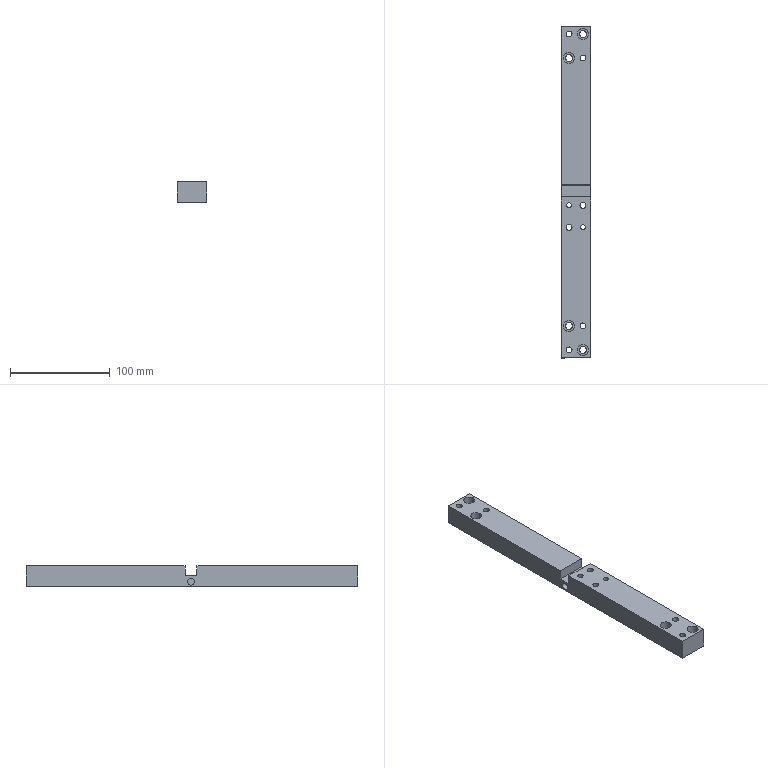Part | NX | features DIE-107 2 | 1 solid | 36 faces | box 30 x 332 x 20.626 mm | volume 191564 mm3 | cylinder 19 | plane 17 | commonest cylinder face diameters 6 x6 7.007 x4 11 x4 5.206 x2 8 x2 7 x1
STEP:
#1=CARTESIAN_POINT('',(4417.594,-1025.122,873.716));
#2=VERTEX_POINT('',#1);
#3=CARTESIAN_POINT('',(4417.594,-693.122,873.716));
#4=VERTEX_POINT('',#3);
#5=CARTESIAN_POINT('',(4417.594,-864.648,873.716));
#6=DIRECTION('',(0.,1.,0.));
#7=VECTOR('',#6,1000.);
#8=LINE('',#5,#7);
#9=EDGE_CURVE('',#2,#4,#8,.T.);
#10=ORIENTED_EDGE('',*,*,#9,.T.);
#11=CARTESIAN_POINT('',(4417.594,-693.122,894.343));
#12=VERTEX_POINT('',#11);
#13=CARTESIAN_POINT('',(4417.594,-693.122,880.343));
#14=DIRECTION('',(0.,0.,1.));
#15=VECTOR('',#14,1000.);
#16=LINE('',#13,#15);
#17=EDGE_CURVE('',#4,#12,#16,.T.);
#18=ORIENTED_EDGE('',*,*,#17,.T.);
#19=CARTESIAN_POINT('',(4417.594,-852.122,894.343));
#20=VERTEX_POINT('',#19);
#21=CARTESIAN_POINT('',(4417.594,-853.596,894.343));
#22=DIRECTION('',(0.,1.,0.));
#23=VECTOR('',#22,1000.);
#24=LINE('',#21,#23);
#25=EDGE_CURVE('',#20,#12,#24,.T.);
#26=ORIENTED_EDGE('',*,*,#25,.F.);
#27=CARTESIAN_POINT('',(4417.594,-852.122,884.343));
#28=VERTEX_POINT('',#27);
#29=CARTESIAN_POINT('',(4417.594,-852.122,902.343));
#30=DIRECTION('',(0.,0.,-1.));
#31=VECTOR('',#30,1000.);
#32=LINE('',#29,#31);
#33=EDGE_CURVE('',#20,#28,#32,.T.);
#34=ORIENTED_EDGE('',*,*,#33,.T.);
#35=CARTESIAN_POINT('',(4417.594,-864.122,884.343));
#36=VERTEX_POINT('',#35);
#37=CARTESIAN_POINT('',(4417.594,-846.122,884.343));
#38=DIRECTION('',(0.,1.,0.));
#39=VECTOR('',#38,1000.);
#40=LINE('',#37,#39);
#41=EDGE_CURVE('',#36,#28,#40,.T.);
#42=ORIENTED_EDGE('',*,*,#41,.F.);
#43=CARTESIAN_POINT('',(4417.594,-864.122,894.343));
#44=VERTEX_POINT('',#43);
#45=CARTESIAN_POINT('',(4417.594,-864.122,902.343));
#46=DIRECTION('',(0.,0.,-1.));
#47=VECTOR('',#46,1000.);
#48=LINE('',#45,#47);
#49=EDGE_CURVE('',#44,#36,#48,.T.);
#50=ORIENTED_EDGE('',*,*,#49,.F.);
#51=CARTESIAN_POINT('',(4417.594,-1025.122,894.343));
#52=VERTEX_POINT('',#51);
#53=CARTESIAN_POINT('',(4417.594,-864.648,894.343));
#54=DIRECTION('',(0.,-1.,0.));
#55=VECTOR('',#54,1000.);
#56=LINE('',#53,#55);
#57=EDGE_CURVE('',#44,#52,#56,.T.);
#58=ORIENTED_EDGE('',*,*,#57,.T.);
#59=CARTESIAN_POINT('',(4417.594,-1025.122,880.343));
#60=DIRECTION('',(0.,0.,1.));
#61=VECTOR('',#60,1000.);
#62=LINE('',#59,#61);
#63=EDGE_CURVE('',#2,#52,#62,.T.);
#64=ORIENTED_EDGE('',*,*,#63,.F.);
#65=EDGE_LOOP('',(#10,#18,#26,#34,#42,#50,#58,#64));
#66=FACE_BOUND('',#65,.T.);
#67=CARTESIAN_POINT('',(4417.594,-864.648,880.343));
#68=DIRECTION('',(1.,0.,0.));
#69=DIRECTION('',(0.,0.,1.));
#70=AXIS2_PLACEMENT_3D('',#67,#68,#69);
#71=PLANE('',#70);
#72=ADVANCED_FACE('',(#66),#71,.T.);
#73=CARTESIAN_POINT('',(4387.594,-858.122,881.843));
#74=VERTEX_POINT('',#73);
#75=CARTESIAN_POINT('',(4387.594,-858.122,878.343));
#76=DIRECTION('',(-1.,0.,0.));
#77=DIRECTION('',(0.,0.,1.));
#78=AXIS2_PLACEMENT_3D('',#75,#76,#77);
#79=CIRCLE('',#78,3.5);
#80=EDGE_CURVE('',#74,#74,#79,.T.);
#81=ORIENTED_EDGE('',*,*,#80,.F.);
#82=EDGE_LOOP('',(#81));
#83=FACE_BOUND('',#82,.T.);
#84=CARTESIAN_POINT('',(4387.594,-693.122,894.343));
#85=VERTEX_POINT('',#84);
#86=CARTESIAN_POINT('',(4387.594,-852.122,894.343));
#87=VERTEX_POINT('',#86);
#88=CARTESIAN_POINT('',(4387.594,-853.596,894.343));
#89=DIRECTION('',(0.,-1.,0.));
#90=VECTOR('',#89,1000.);
#91=LINE('',#88,#90);
#92=EDGE_CURVE('',#85,#87,#91,.T.);
#93=ORIENTED_EDGE('',*,*,#92,.F.);
#94=CARTESIAN_POINT('',(4387.594,-693.122,873.716));
#95=VERTEX_POINT('',#94);
#96=CARTESIAN_POINT('',(4387.594,-693.122,880.343));
#97=DIRECTION('',(0.,0.,-1.));
#98=VECTOR('',#97,1000.);
#99=LINE('',#96,#98);
#100=EDGE_CURVE('',#85,#95,#99,.T.);
#101=ORIENTED_EDGE('',*,*,#100,.T.);
#102=CARTESIAN_POINT('',(4387.594,-1025.122,873.716));
#103=VERTEX_POINT('',#102);
#104=CARTESIAN_POINT('',(4387.594,-864.648,873.716));
#105=DIRECTION('',(0.,-1.,0.));
#106=VECTOR('',#105,1000.);
#107=LINE('',#104,#106);
#108=EDGE_CURVE('',#95,#103,#107,.T.);
#109=ORIENTED_EDGE('',*,*,#108,.T.);
#110=CARTESIAN_POINT('',(4387.594,-1025.122,894.343));
#111=VERTEX_POINT('',#110);
#112=CARTESIAN_POINT('',(4387.594,-1025.122,880.343));
#113=DIRECTION('',(0.,0.,-1.));
#114=VECTOR('',#113,1000.);
#115=LINE('',#112,#114);
#116=EDGE_CURVE('',#111,#103,#115,.T.);
#117=ORIENTED_EDGE('',*,*,#116,.F.);
#118=CARTESIAN_POINT('',(4387.594,-864.122,894.343));
#119=VERTEX_POINT('',#118);
#120=CARTESIAN_POINT('',(4387.594,-864.648,894.343));
#121=DIRECTION('',(0.,1.,0.));
#122=VECTOR('',#121,1000.);
#123=LINE('',#120,#122);
#124=EDGE_CURVE('',#111,#119,#123,.T.);
#125=ORIENTED_EDGE('',*,*,#124,.T.);
#126=CARTESIAN_POINT('',(4387.594,-864.122,884.343));
#127=VERTEX_POINT('',#126);
#128=CARTESIAN_POINT('',(4387.594,-864.122,902.343));
#129=DIRECTION('',(0.,0.,1.));
#130=VECTOR('',#129,1000.);
#131=LINE('',#128,#130);
#132=EDGE_CURVE('',#127,#119,#131,.T.);
#133=ORIENTED_EDGE('',*,*,#132,.F.);
#134=CARTESIAN_POINT('',(4387.594,-852.122,884.343));
#135=VERTEX_POINT('',#134);
#136=CARTESIAN_POINT('',(4387.594,-858.122,884.343));
#137=DIRECTION('',(0.,-1.,0.));
#138=VECTOR('',#137,1000.);
#139=LINE('',#136,#138);
#140=EDGE_CURVE('',#135,#127,#139,.T.);
#141=ORIENTED_EDGE('',*,*,#140,.F.);
#142=CARTESIAN_POINT('',(4387.594,-852.122,902.343));
#143=DIRECTION('',(0.,0.,1.));
#144=VECTOR('',#143,1000.);
#145=LINE('',#142,#144);
#146=EDGE_CURVE('',#135,#87,#145,.T.);
#147=ORIENTED_EDGE('',*,*,#146,.T.);
#148=EDGE_LOOP('',(#93,#101,#109,#117,#125,#133,#141,#147));
#149=FACE_BOUND('',#148,.T.);
#150=CARTESIAN_POINT('',(4387.594,-864.648,880.343));
#151=DIRECTION('',(-1.,0.,0.));
#152=DIRECTION('',(0.,0.,-1.));
#153=AXIS2_PLACEMENT_3D('',#150,#151,#152);
#154=PLANE('',#153);
#155=ADVANCED_FACE('',(#83,#149),#154,.T.);
#156=CARTESIAN_POINT('',(4398.197,-872.372,873.716));
#157=VERTEX_POINT('',#156);
#158=CARTESIAN_POINT('',(4395.594,-872.372,873.716));
#159=DIRECTION('',(0.,0.,1.));
#160=DIRECTION('',(1.,0.,0.));
#161=AXIS2_PLACEMENT_3D('',#158,#159,#160);
#162=CIRCLE('',#161,2.603);
#163=EDGE_CURVE('',#157,#157,#162,.T.);
#164=ORIENTED_EDGE('',*,*,#163,.T.);
#165=EDGE_LOOP('',(#164));
#166=FACE_BOUND('',#165,.T.);
#167=CARTESIAN_POINT('',(4412.197,-894.372,873.716));
#168=VERTEX_POINT('',#167);
#169=CARTESIAN_POINT('',(4409.594,-894.372,873.716));
#170=DIRECTION('',(0.,0.,1.));
#171=DIRECTION('',(1.,0.,0.));
#172=AXIS2_PLACEMENT_3D('',#169,#170,#171);
#173=CIRCLE('',#172,2.603);
#174=EDGE_CURVE('',#168,#168,#173,.T.);
#175=ORIENTED_EDGE('',*,*,#174,.T.);
#176=EDGE_LOOP('',(#175));
#177=FACE_BOUND('',#176,.T.);
#178=CARTESIAN_POINT('',(4413.594,-872.372,873.716));
#179=VERTEX_POINT('',#178);
#180=CARTESIAN_POINT('',(4409.594,-872.372,873.716));
#181=DIRECTION('',(0.,0.,1.));
#182=DIRECTION('',(1.,0.,0.));
#183=AXIS2_PLACEMENT_3D('',#180,#181,#182);
#184=CIRCLE('',#183,4.);
#185=EDGE_CURVE('',#179,#179,#184,.T.);
#186=ORIENTED_EDGE('',*,*,#185,.T.);
#187=EDGE_LOOP('',(#186));
#188=FACE_BOUND('',#187,.T.);
#189=CARTESIAN_POINT('',(4399.594,-894.372,873.716));
#190=VERTEX_POINT('',#189);
#191=CARTESIAN_POINT('',(4395.594,-894.372,873.716));
#192=DIRECTION('',(0.,0.,1.));
#193=DIRECTION('',(1.,0.,0.));
#194=AXIS2_PLACEMENT_3D('',#191,#192,#193);
#195=CIRCLE('',#194,4.);
#196=EDGE_CURVE('',#190,#190,#195,.T.);
#197=ORIENTED_EDGE('',*,*,#196,.T.);
#198=EDGE_LOOP('',(#197));
#199=FACE_BOUND('',#198,.T.);
#200=ORIENTED_EDGE('',*,*,#108,.F.);
#201=CARTESIAN_POINT('',(4402.594,-693.122,873.716));
#202=DIRECTION('',(-1.,0.,0.));
#203=VECTOR('',#202,1000.);
#204=LINE('',#201,#203);
#205=EDGE_CURVE('',#4,#95,#204,.T.);
#206=ORIENTED_EDGE('',*,*,#205,.F.);
#207=ORIENTED_EDGE('',*,*,#9,.F.);
#208=CARTESIAN_POINT('',(4402.594,-1025.122,873.716));
#209=DIRECTION('',(-1.,0.,0.));
#210=VECTOR('',#209,1000.);
#211=LINE('',#208,#210);
#212=EDGE_CURVE('',#2,#103,#211,.T.);
#213=ORIENTED_EDGE('',*,*,#212,.T.);
#214=EDGE_LOOP('',(#200,#206,#207,#213));
#215=FACE_BOUND('',#214,.T.);
#216=CARTESIAN_POINT('',(4409.594,-990.122,873.716));
#217=VERTEX_POINT('',#216);
#218=CARTESIAN_POINT('',(4409.594,-993.122,873.716));
#219=DIRECTION('',(0.,0.,1.));
#220=DIRECTION('',(0.,1.,0.));
#221=AXIS2_PLACEMENT_3D('',#218,#219,#220);
#222=CIRCLE('',#221,3.);
#223=EDGE_CURVE('',#217,#217,#222,.T.);
#224=ORIENTED_EDGE('',*,*,#223,.T.);
#225=EDGE_LOOP('',(#224));
#226=FACE_BOUND('',#225,.T.);
#227=CARTESIAN_POINT('',(4395.594,-1014.122,873.716));
#228=VERTEX_POINT('',#227);
#229=CARTESIAN_POINT('',(4395.594,-1017.122,873.716));
#230=DIRECTION('',(0.,0.,1.));
#231=DIRECTION('',(0.,1.,0.));
#232=AXIS2_PLACEMENT_3D('',#229,#230,#231);
#233=CIRCLE('',#232,3.);
#234=EDGE_CURVE('',#228,#228,#233,.T.);
#235=ORIENTED_EDGE('',*,*,#234,.T.);
#236=EDGE_LOOP('',(#235));
#237=FACE_BOUND('',#236,.T.);
#238=CARTESIAN_POINT('',(4395.594,-989.619,873.716));
#239=VERTEX_POINT('',#238);
#240=CARTESIAN_POINT('',(4395.594,-993.122,873.716));
#241=DIRECTION('',(0.,0.,1.));
#242=DIRECTION('',(0.,1.,0.));
#243=AXIS2_PLACEMENT_3D('',#240,#241,#242);
#244=CIRCLE('',#243,3.503);
#245=EDGE_CURVE('',#239,#239,#244,.T.);
#246=ORIENTED_EDGE('',*,*,#245,.T.);
#247=EDGE_LOOP('',(#246));
#248=FACE_BOUND('',#247,.T.);
#249=CARTESIAN_POINT('',(4409.594,-1013.619,873.716));
#250=VERTEX_POINT('',#249);
#251=CARTESIAN_POINT('',(4409.594,-1017.122,873.716));
#252=DIRECTION('',(0.,0.,1.));
#253=DIRECTION('',(0.,1.,0.));
#254=AXIS2_PLACEMENT_3D('',#251,#252,#253);
#255=CIRCLE('',#254,3.503);
#256=EDGE_CURVE('',#250,#250,#255,.T.);
#257=ORIENTED_EDGE('',*,*,#256,.T.);
#258=EDGE_LOOP('',(#257));
#259=FACE_BOUND('',#258,.T.);
#260=CARTESIAN_POINT('',(4409.594,-728.122,873.716));
#261=VERTEX_POINT('',#260);
#262=CARTESIAN_POINT('',(4409.594,-725.122,873.716));
#263=DIRECTION('',(0.,0.,-1.));
#264=DIRECTION('',(0.,-1.,0.));
#265=AXIS2_PLACEMENT_3D('',#262,#263,#264);
#266=CIRCLE('',#265,3.);
#267=EDGE_CURVE('',#261,#261,#266,.T.);
#268=ORIENTED_EDGE('',*,*,#267,.F.);
#269=EDGE_LOOP('',(#268));
#270=FACE_BOUND('',#269,.T.);
#271=CARTESIAN_POINT('',(4395.594,-704.122,873.716));
#272=VERTEX_POINT('',#271);
#273=CARTESIAN_POINT('',(4395.594,-701.122,873.716));
#274=DIRECTION('',(0.,0.,-1.));
#275=DIRECTION('',(0.,-1.,0.));
#276=AXIS2_PLACEMENT_3D('',#273,#274,#275);
#277=CIRCLE('',#276,3.);
#278=EDGE_CURVE('',#272,#272,#277,.T.);
#279=ORIENTED_EDGE('',*,*,#278,.F.);
#280=EDGE_LOOP('',(#279));
#281=FACE_BOUND('',#280,.T.);
#282=CARTESIAN_POINT('',(4395.594,-728.626,873.716));
#283=VERTEX_POINT('',#282);
#284=CARTESIAN_POINT('',(4395.594,-725.122,873.716));
#285=DIRECTION('',(0.,0.,-1.));
#286=DIRECTION('',(0.,-1.,0.));
#287=AXIS2_PLACEMENT_3D('',#284,#285,#286);
#288=CIRCLE('',#287,3.503);
#289=EDGE_CURVE('',#283,#283,#288,.T.);
#290=ORIENTED_EDGE('',*,*,#289,.F.);
#291=EDGE_LOOP('',(#290));
#292=FACE_BOUND('',#291,.T.);
#293=CARTESIAN_POINT('',(4409.594,-704.626,873.716));
#294=VERTEX_POINT('',#293);
#295=CARTESIAN_POINT('',(4409.594,-701.122,873.716));
#296=DIRECTION('',(0.,0.,-1.));
#297=DIRECTION('',(0.,-1.,0.));
#298=AXIS2_PLACEMENT_3D('',#295,#296,#297);
#299=CIRCLE('',#298,3.503);
#300=EDGE_CURVE('',#294,#294,#299,.T.);
#301=ORIENTED_EDGE('',*,*,#300,.F.);
#302=EDGE_LOOP('',(#301));
#303=FACE_BOUND('',#302,.T.);
#304=CARTESIAN_POINT('',(3639.721,-859.122,873.716));
#305=DIRECTION('',(0.,0.,1.));
#306=DIRECTION('',(1.,0.,0.));
#307=AXIS2_PLACEMENT_3D('',#304,#305,#306);
#308=PLANE('',#307);
#309=ADVANCED_FACE('',(#166,#177,#188,#199,#215,#226,#237,#248,#259,#270,#281,#292,#303),#308,.F.);
#310=ORIENTED_EDGE('',*,*,#25,.T.);
#311=CARTESIAN_POINT('',(4386.594,-693.122,894.343));
#312=DIRECTION('',(-1.,0.,0.));
#313=VECTOR('',#312,1000.);
#314=LINE('',#311,#313);
#315=EDGE_CURVE('',#12,#85,#314,.T.);
#316=ORIENTED_EDGE('',*,*,#315,.T.);
#317=ORIENTED_EDGE('',*,*,#92,.T.);
#318=CARTESIAN_POINT('',(4409.594,-852.122,894.343));
#319=DIRECTION('',(1.,0.,0.));
#320=VECTOR('',#319,1000.);
#321=LINE('',#318,#320);
#322=EDGE_CURVE('',#87,#20,#321,.T.);
#323=ORIENTED_EDGE('',*,*,#322,.T.);
#324=EDGE_LOOP('',(#310,#316,#317,#323));
#325=FACE_BOUND('',#324,.T.);
#326=CARTESIAN_POINT('',(4412.594,-725.122,894.343));
#327=VERTEX_POINT('',#326);
#328=CARTESIAN_POINT('',(4409.594,-725.122,894.343));
#329=DIRECTION('',(0.,0.,-1.));
#330=DIRECTION('',(1.,0.,0.));
#331=AXIS2_PLACEMENT_3D('',#328,#329,#330);
#332=CIRCLE('',#331,3.);
#333=EDGE_CURVE('',#327,#327,#332,.T.);
#334=ORIENTED_EDGE('',*,*,#333,.T.);
#335=EDGE_LOOP('',(#334));
#336=FACE_BOUND('',#335,.T.);
#337=CARTESIAN_POINT('',(4398.594,-701.122,894.343));
#338=VERTEX_POINT('',#337);
#339=CARTESIAN_POINT('',(4395.594,-701.122,894.343));
#340=DIRECTION('',(0.,0.,-1.));
#341=DIRECTION('',(1.,0.,0.));
#342=AXIS2_PLACEMENT_3D('',#339,#340,#341);
#343=CIRCLE('',#342,3.);
#344=EDGE_CURVE('',#338,#338,#343,.T.);
#345=ORIENTED_EDGE('',*,*,#344,.T.);
#346=EDGE_LOOP('',(#345));
#347=FACE_BOUND('',#346,.T.);
#348=CARTESIAN_POINT('',(4401.094,-725.122,894.343));
#349=VERTEX_POINT('',#348);
#350=CARTESIAN_POINT('',(4395.594,-725.122,894.343));
#351=DIRECTION('',(0.,0.,-1.));
#352=DIRECTION('',(1.,0.,0.));
#353=AXIS2_PLACEMENT_3D('',#350,#351,#352);
#354=CIRCLE('',#353,5.5);
#355=EDGE_CURVE('',#349,#349,#354,.T.);
#356=ORIENTED_EDGE('',*,*,#355,.T.);
#357=EDGE_LOOP('',(#356));
#358=FACE_BOUND('',#357,.T.);
#359=CARTESIAN_POINT('',(4415.094,-701.122,894.343));
#360=VERTEX_POINT('',#359);
#361=CARTESIAN_POINT('',(4409.594,-701.122,894.343));
#362=DIRECTION('',(0.,0.,-1.));
#363=DIRECTION('',(1.,0.,0.));
#364=AXIS2_PLACEMENT_3D('',#361,#362,#363);
#365=CIRCLE('',#364,5.5);
#366=EDGE_CURVE('',#360,#360,#365,.T.);
#367=ORIENTED_EDGE('',*,*,#366,.T.);
#368=EDGE_LOOP('',(#367));
#369=FACE_BOUND('',#368,.T.);
#370=CARTESIAN_POINT('',(4386.594,-830.596,894.343));
#371=DIRECTION('',(0.,0.,1.));
#372=DIRECTION('',(0.,1.,0.));
#373=AXIS2_PLACEMENT_3D('',#370,#371,#372);
#374=PLANE('',#373);
#375=ADVANCED_FACE('',(#325,#336,#347,#358,#369),#374,.T.);
#376=CARTESIAN_POINT('',(4398.197,-872.372,894.343));
#377=VERTEX_POINT('',#376);
#378=CARTESIAN_POINT('',(4395.594,-872.372,894.343));
#379=DIRECTION('',(0.,0.,-1.));
#380=DIRECTION('',(1.,0.,0.));
#381=AXIS2_PLACEMENT_3D('',#378,#379,#380);
#382=CIRCLE('',#381,2.603);
#383=EDGE_CURVE('',#377,#377,#382,.T.);
#384=ORIENTED_EDGE('',*,*,#383,.T.);
#385=EDGE_LOOP('',(#384));
#386=FACE_BOUND('',#385,.T.);
#387=CARTESIAN_POINT('',(4412.197,-894.372,894.343));
#388=VERTEX_POINT('',#387);
#389=CARTESIAN_POINT('',(4409.594,-894.372,894.343));
#390=DIRECTION('',(0.,0.,-1.));
#391=DIRECTION('',(1.,0.,0.));
#392=AXIS2_PLACEMENT_3D('',#389,#390,#391);
#393=CIRCLE('',#392,2.603);
#394=EDGE_CURVE('',#388,#388,#393,.T.);
#395=ORIENTED_EDGE('',*,*,#394,.T.);
#396=EDGE_LOOP('',(#395));
#397=FACE_BOUND('',#396,.T.);
#398=CARTESIAN_POINT('',(4412.594,-872.372,894.343));
#399=VERTEX_POINT('',#398);
#400=CARTESIAN_POINT('',(4409.594,-872.372,894.343));
#401=DIRECTION('',(0.,0.,-1.));
#402=DIRECTION('',(1.,0.,0.));
#403=AXIS2_PLACEMENT_3D('',#400,#401,#402);
#404=CIRCLE('',#403,3.);
#405=EDGE_CURVE('',#399,#399,#404,.T.);
#406=ORIENTED_EDGE('',*,*,#405,.T.);
#407=EDGE_LOOP('',(#406));
#408=FACE_BOUND('',#407,.T.);
#409=CARTESIAN_POINT('',(4398.594,-894.372,894.343));
#410=VERTEX_POINT('',#409);
#411=CARTESIAN_POINT('',(4395.594,-894.372,894.343));
#412=DIRECTION('',(0.,0.,-1.));
#413=DIRECTION('',(1.,0.,0.));
#414=AXIS2_PLACEMENT_3D('',#411,#412,#413);
#415=CIRCLE('',#414,3.);
#416=EDGE_CURVE('',#410,#410,#415,.T.);
#417=ORIENTED_EDGE('',*,*,#416,.T.);
#418=EDGE_LOOP('',(#417));
#419=FACE_BOUND('',#418,.T.);
#420=ORIENTED_EDGE('',*,*,#124,.F.);
#421=CARTESIAN_POINT('',(4386.594,-1025.122,894.343));
#422=DIRECTION('',(-1.,0.,0.));
#423=VECTOR('',#422,1000.);
#424=LINE('',#421,#423);
#425=EDGE_CURVE('',#52,#111,#424,.T.);
#426=ORIENTED_EDGE('',*,*,#425,.F.);
#427=ORIENTED_EDGE('',*,*,#57,.F.);
#428=CARTESIAN_POINT('',(4409.594,-864.122,894.343));
#429=DIRECTION('',(1.,0.,0.));
#430=VECTOR('',#429,1000.);
#431=LINE('',#428,#430);
#432=EDGE_CURVE('',#119,#44,#431,.T.);
#433=ORIENTED_EDGE('',*,*,#432,.F.);
#434=EDGE_LOOP('',(#420,#426,#427,#433));
#435=FACE_BOUND('',#434,.T.);
#436=CARTESIAN_POINT('',(4412.594,-993.122,894.343));
#437=VERTEX_POINT('',#436);
#438=CARTESIAN_POINT('',(4409.594,-993.122,894.343));
#439=DIRECTION('',(0.,0.,1.));
#440=DIRECTION('',(1.,0.,0.));
#441=AXIS2_PLACEMENT_3D('',#438,#439,#440);
#442=CIRCLE('',#441,3.);
#443=EDGE_CURVE('',#437,#437,#442,.T.);
#444=ORIENTED_EDGE('',*,*,#443,.F.);
#445=EDGE_LOOP('',(#444));
#446=FACE_BOUND('',#445,.T.);
#447=CARTESIAN_POINT('',(4398.594,-1017.122,894.343));
#448=VERTEX_POINT('',#447);
#449=CARTESIAN_POINT('',(4395.594,-1017.122,894.343));
#450=DIRECTION('',(0.,0.,1.));
#451=DIRECTION('',(1.,0.,0.));
#452=AXIS2_PLACEMENT_3D('',#449,#450,#451);
#453=CIRCLE('',#452,3.);
#454=EDGE_CURVE('',#448,#448,#453,.T.);
#455=ORIENTED_EDGE('',*,*,#454,.F.);
#456=EDGE_LOOP('',(#455));
#457=FACE_BOUND('',#456,.T.);
#458=CARTESIAN_POINT('',(4401.094,-993.122,894.343));
#459=VERTEX_POINT('',#458);
#460=CARTESIAN_POINT('',(4395.594,-993.122,894.343));
#461=DIRECTION('',(0.,0.,1.));
#462=DIRECTION('',(1.,0.,0.));
#463=AXIS2_PLACEMENT_3D('',#460,#461,#462);
#464=CIRCLE('',#463,5.5);
#465=EDGE_CURVE('',#459,#459,#464,.T.);
#466=ORIENTED_EDGE('',*,*,#465,.F.);
#467=EDGE_LOOP('',(#466));
#468=FACE_BOUND('',#467,.T.);
#469=CARTESIAN_POINT('',(4415.094,-1017.122,894.343));
#470=VERTEX_POINT('',#469);
#471=CARTESIAN_POINT('',(4409.594,-1017.122,894.343));
#472=DIRECTION('',(0.,0.,1.));
#473=DIRECTION('',(1.,0.,0.));
#474=AXIS2_PLACEMENT_3D('',#471,#472,#473);
#475=CIRCLE('',#474,5.5);
#476=EDGE_CURVE('',#470,#470,#475,.T.);
#477=ORIENTED_EDGE('',*,*,#476,.F.);
#478=EDGE_LOOP('',(#477));
#479=FACE_BOUND('',#478,.T.);
#480=CARTESIAN_POINT('',(4386.594,-887.648,894.343));
#481=DIRECTION('',(0.,0.,1.));
#482=DIRECTION('',(0.,-1.,0.));
#483=AXIS2_PLACEMENT_3D('',#480,#481,#482);
#484=PLANE('',#483);
#485=ADVANCED_FACE('',(#386,#397,#408,#419,#435,#446,#457,#468,#479),#484,.T.);
#486=CARTESIAN_POINT('',(4404.594,-858.122,881.843));
#487=VERTEX_POINT('',#486);
#488=CARTESIAN_POINT('',(4404.594,-858.122,878.343));
#489=DIRECTION('',(1.,0.,0.));
#490=DIRECTION('',(0.,0.,1.));
#491=AXIS2_PLACEMENT_3D('',#488,#489,#490);
#492=CIRCLE('',#491,3.5);
#493=EDGE_CURVE('',#487,#487,#492,.T.);
#494=ORIENTED_EDGE('',*,*,#493,.F.);
#495=EDGE_LOOP('',(#494));
#496=FACE_BOUND('',#495,.T.);
#497=CARTESIAN_POINT('',(4404.594,-846.122,882.343));
#498=DIRECTION('',(-1.,0.,0.));
#499=DIRECTION('',(0.,0.,-1.));
#500=AXIS2_PLACEMENT_3D('',#497,#498,#499);
#501=PLANE('',#500);
#502=ADVANCED_FACE('',(#496),#501,.T.);
#503=ORIENTED_EDGE('',*,*,#80,.T.);
#504=EDGE_LOOP('',(#503));
#505=FACE_BOUND('',#504,.T.);
#506=ORIENTED_EDGE('',*,*,#493,.T.);
#507=EDGE_LOOP('',(#506));
#508=FACE_BOUND('',#507,.T.);
#509=CARTESIAN_POINT('',(4374.594,-858.122,878.343));
#510=DIRECTION('',(-1.,0.,0.));
#511=DIRECTION('',(0.,-1.,0.));
#512=AXIS2_PLACEMENT_3D('',#509,#510,#511);
#513=CYLINDRICAL_SURFACE('',#512,3.5);
#514=ADVANCED_FACE('',(#505,#508),#513,.F.);
#515=ORIENTED_EDGE('',*,*,#41,.T.);
#516=CARTESIAN_POINT('',(4409.594,-852.122,884.343));
#517=DIRECTION('',(1.,0.,0.));
#518=VECTOR('',#517,1000.);
#519=LINE('',#516,#518);
#520=EDGE_CURVE('',#135,#28,#519,.T.);
#521=ORIENTED_EDGE('',*,*,#520,.F.);
#522=ORIENTED_EDGE('',*,*,#140,.T.);
#523=CARTESIAN_POINT('',(4409.594,-864.122,884.343));
#524=DIRECTION('',(1.,0.,0.));
#525=VECTOR('',#524,1000.);
#526=LINE('',#523,#525);
#527=EDGE_CURVE('',#127,#36,#526,.T.);
#528=ORIENTED_EDGE('',*,*,#527,.T.);
#529=EDGE_LOOP('',(#515,#521,#522,#528));
#530=FACE_BOUND('',#529,.T.);
#531=CARTESIAN_POINT('',(4366.094,-858.122,884.343));
#532=DIRECTION('',(0.,0.,1.));
#533=DIRECTION('',(0.,1.,0.));
#534=AXIS2_PLACEMENT_3D('',#531,#532,#533);
#535=PLANE('',#534);
#536=ADVANCED_FACE('',(#530),#535,.T.);
#537=ORIENTED_EDGE('',*,*,#527,.F.);
#538=ORIENTED_EDGE('',*,*,#132,.T.);
#539=ORIENTED_EDGE('',*,*,#432,.T.);
#540=ORIENTED_EDGE('',*,*,#49,.T.);
#541=EDGE_LOOP('',(#537,#538,#539,#540));
#542=FACE_BOUND('',#541,.T.);
#543=CARTESIAN_POINT('',(4409.594,-864.122,902.343));
#544=DIRECTION('',(0.,1.,0.));
#545=DIRECTION('',(0.,0.,1.));
#546=AXIS2_PLACEMENT_3D('',#543,#544,#545);
#547=PLANE('',#546);
#548=ADVANCED_FACE('',(#542),#547,.T.);
#549=ORIENTED_EDGE('',*,*,#520,.T.);
#550=ORIENTED_EDGE('',*,*,#33,.F.);
#551=ORIENTED_EDGE('',*,*,#322,.F.);
#552=ORIENTED_EDGE('',*,*,#146,.F.);
#553=EDGE_LOOP('',(#549,#550,#551,#552));
#554=FACE_BOUND('',#553,.T.);
#555=CARTESIAN_POINT('',(4409.594,-852.122,902.343));
#556=DIRECTION('',(0.,-1.,0.));
#557=DIRECTION('',(0.,0.,1.));
#558=AXIS2_PLACEMENT_3D('',#555,#556,#557);
#559=PLANE('',#558);
#560=ADVANCED_FACE('',(#554),#559,.T.);
#561=ORIENTED_EDGE('',*,*,#212,.F.);
#562=ORIENTED_EDGE('',*,*,#63,.T.);
#563=ORIENTED_EDGE('',*,*,#425,.T.);
#564=ORIENTED_EDGE('',*,*,#116,.T.);
#565=EDGE_LOOP('',(#561,#562,#563,#564));
#566=FACE_BOUND('',#565,.T.);
#567=CARTESIAN_POINT('',(4402.594,-1025.122,845.029));
#568=DIRECTION('',(0.,1.,0.));
#569=DIRECTION('',(0.,0.,-1.));
#570=AXIS2_PLACEMENT_3D('',#567,#568,#569);
#571=PLANE('',#570);
#572=ADVANCED_FACE('',(#566),#571,.F.);
#573=ORIENTED_EDGE('',*,*,#256,.F.);
#574=EDGE_LOOP('',(#573));
#575=FACE_BOUND('',#574,.T.);
#576=CARTESIAN_POINT('',(4413.097,-1017.122,885.343));
#577=VERTEX_POINT('',#576);
#578=CARTESIAN_POINT('',(4409.594,-1017.122,885.343));
#579=DIRECTION('',(0.,0.,1.));
#580=DIRECTION('',(1.,0.,0.));
#581=AXIS2_PLACEMENT_3D('',#578,#579,#580);
#582=CIRCLE('',#581,3.503);
#583=EDGE_CURVE('',#577,#577,#582,.T.);
#584=ORIENTED_EDGE('',*,*,#583,.T.);
#585=EDGE_LOOP('',(#584));
#586=FACE_BOUND('',#585,.T.);
#587=CARTESIAN_POINT('',(4409.594,-1017.122,873.716));
#588=DIRECTION('',(0.,0.,1.));
#589=DIRECTION('',(-1.,0.,0.));
#590=AXIS2_PLACEMENT_3D('',#587,#588,#589);
#591=CYLINDRICAL_SURFACE('',#590,3.503);
#592=ADVANCED_FACE('',(#575,#586),#591,.F.);
#593=ORIENTED_EDGE('',*,*,#476,.T.);
#594=EDGE_LOOP('',(#593));
#595=FACE_BOUND('',#594,.T.);
#596=CARTESIAN_POINT('',(4409.594,-1011.622,885.343));
#597=VERTEX_POINT('',#596);
#598=CARTESIAN_POINT('',(4409.594,-1017.122,885.343));
#599=DIRECTION('',(0.,0.,-1.));
#600=DIRECTION('',(0.,1.,0.));
#601=AXIS2_PLACEMENT_3D('',#598,#599,#600);
#602=CIRCLE('',#601,5.5);
#603=EDGE_CURVE('',#597,#597,#602,.T.);
#604=ORIENTED_EDGE('',*,*,#603,.T.);
#605=EDGE_LOOP('',(#604));
#606=FACE_BOUND('',#605,.T.);
#607=CARTESIAN_POINT('',(4409.594,-1017.122,885.343));
#608=DIRECTION('',(0.,0.,1.));
#609=DIRECTION('',(-1.,0.,0.));
#610=AXIS2_PLACEMENT_3D('',#607,#608,#609);
#611=CYLINDRICAL_SURFACE('',#610,5.5);
#612=ADVANCED_FACE('',(#595,#606),#611,.F.);
#613=ORIENTED_EDGE('',*,*,#583,.F.);
#614=EDGE_LOOP('',(#613));
#615=FACE_BOUND('',#614,.T.);
#616=ORIENTED_EDGE('',*,*,#603,.F.);
#617=EDGE_LOOP('',(#616));
#618=FACE_BOUND('',#617,.T.);
#619=CARTESIAN_POINT('',(4409.594,-1017.122,885.343));
#620=DIRECTION('',(0.,0.,1.));
#621=DIRECTION('',(-1.,0.,0.));
#622=AXIS2_PLACEMENT_3D('',#619,#620,#621);
#623=PLANE('',#622);
#624=ADVANCED_FACE('',(#615,#618),#623,.T.);
#625=ORIENTED_EDGE('',*,*,#245,.F.);
#626=EDGE_LOOP('',(#625));
#627=FACE_BOUND('',#626,.T.);
#628=CARTESIAN_POINT('',(4399.097,-993.122,885.343));
#629=VERTEX_POINT('',#628);
#630=CARTESIAN_POINT('',(4395.594,-993.122,885.343));
#631=DIRECTION('',(0.,0.,1.));
#632=DIRECTION('',(1.,0.,0.));
#633=AXIS2_PLACEMENT_3D('',#630,#631,#632);
#634=CIRCLE('',#633,3.503);
#635=EDGE_CURVE('',#629,#629,#634,.T.);
#636=ORIENTED_EDGE('',*,*,#635,.T.);
#637=EDGE_LOOP('',(#636));
#638=FACE_BOUND('',#637,.T.);
#639=CARTESIAN_POINT('',(4395.594,-993.122,873.716));
#640=DIRECTION('',(0.,0.,1.));
#641=DIRECTION('',(-1.,0.,0.));
#642=AXIS2_PLACEMENT_3D('',#639,#640,#641);
#643=CYLINDRICAL_SURFACE('',#642,3.503);
#644=ADVANCED_FACE('',(#627,#638),#643,.F.);
#645=ORIENTED_EDGE('',*,*,#465,.T.);
#646=EDGE_LOOP('',(#645));
#647=FACE_BOUND('',#646,.T.);
#648=CARTESIAN_POINT('',(4395.594,-987.622,885.343));
#649=VERTEX_POINT('',#648);
#650=CARTESIAN_POINT('',(4395.594,-993.122,885.343));
#651=DIRECTION('',(0.,0.,-1.));
#652=DIRECTION('',(0.,1.,0.));
#653=AXIS2_PLACEMENT_3D('',#650,#651,#652);
#654=CIRCLE('',#653,5.5);
#655=EDGE_CURVE('',#649,#649,#654,.T.);
#656=ORIENTED_EDGE('',*,*,#655,.T.);
#657=EDGE_LOOP('',(#656));
#658=FACE_BOUND('',#657,.T.);
#659=CARTESIAN_POINT('',(4395.594,-993.122,885.343));
#660=DIRECTION('',(0.,0.,1.));
#661=DIRECTION('',(-1.,0.,0.));
#662=AXIS2_PLACEMENT_3D('',#659,#660,#661);
#663=CYLINDRICAL_SURFACE('',#662,5.5);
#664=ADVANCED_FACE('',(#647,#658),#663,.F.);
#665=ORIENTED_EDGE('',*,*,#635,.F.);
#666=EDGE_LOOP('',(#665));
#667=FACE_BOUND('',#666,.T.);
#668=ORIENTED_EDGE('',*,*,#655,.F.);
#669=EDGE_LOOP('',(#668));
#670=FACE_BOUND('',#669,.T.);
#671=CARTESIAN_POINT('',(4395.594,-993.122,885.343));
#672=DIRECTION('',(0.,0.,1.));
#673=DIRECTION('',(-1.,0.,0.));
#674=AXIS2_PLACEMENT_3D('',#671,#672,#673);
#675=PLANE('',#674);
#676=ADVANCED_FACE('',(#667,#670),#675,.T.);
#677=ORIENTED_EDGE('',*,*,#454,.T.);
#678=EDGE_LOOP('',(#677));
#679=FACE_BOUND('',#678,.T.);
#680=ORIENTED_EDGE('',*,*,#234,.F.);
#681=EDGE_LOOP('',(#680));
#682=FACE_BOUND('',#681,.T.);
#683=CARTESIAN_POINT('',(4395.594,-1017.122,873.716));
#684=DIRECTION('',(0.,0.,1.));
#685=DIRECTION('',(-1.,0.,0.));
#686=AXIS2_PLACEMENT_3D('',#683,#684,#685);
#687=CYLINDRICAL_SURFACE('',#686,3.);
#688=ADVANCED_FACE('',(#679,#682),#687,.F.);
#689=ORIENTED_EDGE('',*,*,#443,.T.);
#690=EDGE_LOOP('',(#689));
#691=FACE_BOUND('',#690,.T.);
#692=ORIENTED_EDGE('',*,*,#223,.F.);
#693=EDGE_LOOP('',(#692));
#694=FACE_BOUND('',#693,.T.);
#695=CARTESIAN_POINT('',(4409.594,-993.122,873.716));
#696=DIRECTION('',(0.,0.,1.));
#697=DIRECTION('',(-1.,0.,0.));
#698=AXIS2_PLACEMENT_3D('',#695,#696,#697);
#699=CYLINDRICAL_SURFACE('',#698,3.);
#700=ADVANCED_FACE('',(#691,#694),#699,.F.);
#701=ORIENTED_EDGE('',*,*,#205,.T.);
#702=ORIENTED_EDGE('',*,*,#100,.F.);
#703=ORIENTED_EDGE('',*,*,#315,.F.);
#704=ORIENTED_EDGE('',*,*,#17,.F.);
#705=EDGE_LOOP('',(#701,#702,#703,#704));
#706=FACE_BOUND('',#705,.T.);
#707=CARTESIAN_POINT('',(4402.594,-693.122,845.029));
#708=DIRECTION('',(0.,-1.,0.));
#709=DIRECTION('',(0.,0.,-1.));
#710=AXIS2_PLACEMENT_3D('',#707,#708,#709);
#711=PLANE('',#710);
#712=ADVANCED_FACE('',(#706),#711,.F.);
#713=ORIENTED_EDGE('',*,*,#300,.T.);
#714=EDGE_LOOP('',(#713));
#715=FACE_BOUND('',#714,.T.);
#716=CARTESIAN_POINT('',(4413.097,-701.122,885.343));
#717=VERTEX_POINT('',#716);
#718=CARTESIAN_POINT('',(4409.594,-701.122,885.343));
#719=DIRECTION('',(0.,0.,-1.));
#720=DIRECTION('',(1.,0.,0.));
#721=AXIS2_PLACEMENT_3D('',#718,#719,#720);
#722=CIRCLE('',#721,3.503);
#723=EDGE_CURVE('',#717,#717,#722,.T.);
#724=ORIENTED_EDGE('',*,*,#723,.F.);
#725=EDGE_LOOP('',(#724));
#726=FACE_BOUND('',#725,.T.);
#727=CARTESIAN_POINT('',(4409.594,-701.122,873.716));
#728=DIRECTION('',(0.,0.,1.));
#729=DIRECTION('',(-1.,0.,0.));
#730=AXIS2_PLACEMENT_3D('',#727,#728,#729);
#731=CYLINDRICAL_SURFACE('',#730,3.503);
#732=ADVANCED_FACE('',(#715,#726),#731,.F.);
#733=ORIENTED_EDGE('',*,*,#366,.F.);
#734=EDGE_LOOP('',(#733));
#735=FACE_BOUND('',#734,.T.);
#736=CARTESIAN_POINT('',(4409.594,-706.622,885.343));
#737=VERTEX_POINT('',#736);
#738=CARTESIAN_POINT('',(4409.594,-701.122,885.343));
#739=DIRECTION('',(0.,0.,1.));
#740=DIRECTION('',(0.,-1.,0.));
#741=AXIS2_PLACEMENT_3D('',#738,#739,#740);
#742=CIRCLE('',#741,5.5);
#743=EDGE_CURVE('',#737,#737,#742,.T.);
#744=ORIENTED_EDGE('',*,*,#743,.F.);
#745=EDGE_LOOP('',(#744));
#746=FACE_BOUND('',#745,.T.);
#747=CARTESIAN_POINT('',(4409.594,-701.122,885.343));
#748=DIRECTION('',(0.,0.,1.));
#749=DIRECTION('',(-1.,0.,0.));
#750=AXIS2_PLACEMENT_3D('',#747,#748,#749);
#751=CYLINDRICAL_SURFACE('',#750,5.5);
#752=ADVANCED_FACE('',(#735,#746),#751,.F.);
#753=ORIENTED_EDGE('',*,*,#723,.T.);
#754=EDGE_LOOP('',(#753));
#755=FACE_BOUND('',#754,.T.);
#756=ORIENTED_EDGE('',*,*,#743,.T.);
#757=EDGE_LOOP('',(#756));
#758=FACE_BOUND('',#757,.T.);
#759=CARTESIAN_POINT('',(4409.594,-701.122,885.343));
#760=DIRECTION('',(0.,0.,1.));
#761=DIRECTION('',(-1.,0.,0.));
#762=AXIS2_PLACEMENT_3D('',#759,#760,#761);
#763=PLANE('',#762);
#764=ADVANCED_FACE('',(#755,#758),#763,.T.);
#765=ORIENTED_EDGE('',*,*,#289,.T.);
#766=EDGE_LOOP('',(#765));
#767=FACE_BOUND('',#766,.T.);
#768=CARTESIAN_POINT('',(4399.097,-725.122,885.343));
#769=VERTEX_POINT('',#768);
#770=CARTESIAN_POINT('',(4395.594,-725.122,885.343));
#771=DIRECTION('',(0.,0.,-1.));
#772=DIRECTION('',(1.,0.,0.));
#773=AXIS2_PLACEMENT_3D('',#770,#771,#772);
#774=CIRCLE('',#773,3.503);
#775=EDGE_CURVE('',#769,#769,#774,.T.);
#776=ORIENTED_EDGE('',*,*,#775,.F.);
#777=EDGE_LOOP('',(#776));
#778=FACE_BOUND('',#777,.T.);
#779=CARTESIAN_POINT('',(4395.594,-725.122,873.716));
#780=DIRECTION('',(0.,0.,1.));
#781=DIRECTION('',(-1.,0.,0.));
#782=AXIS2_PLACEMENT_3D('',#779,#780,#781);
#783=CYLINDRICAL_SURFACE('',#782,3.503);
#784=ADVANCED_FACE('',(#767,#778),#783,.F.);
#785=ORIENTED_EDGE('',*,*,#355,.F.);
#786=EDGE_LOOP('',(#785));
#787=FACE_BOUND('',#786,.T.);
#788=CARTESIAN_POINT('',(4395.594,-730.622,885.343));
#789=VERTEX_POINT('',#788);
#790=CARTESIAN_POINT('',(4395.594,-725.122,885.343));
#791=DIRECTION('',(0.,0.,1.));
#792=DIRECTION('',(0.,-1.,0.));
#793=AXIS2_PLACEMENT_3D('',#790,#791,#792);
#794=CIRCLE('',#793,5.5);
#795=EDGE_CURVE('',#789,#789,#794,.T.);
#796=ORIENTED_EDGE('',*,*,#795,.F.);
#797=EDGE_LOOP('',(#796));
#798=FACE_BOUND('',#797,.T.);
#799=CARTESIAN_POINT('',(4395.594,-725.122,885.343));
#800=DIRECTION('',(0.,0.,1.));
#801=DIRECTION('',(-1.,0.,0.));
#802=AXIS2_PLACEMENT_3D('',#799,#800,#801);
#803=CYLINDRICAL_SURFACE('',#802,5.5);
#804=ADVANCED_FACE('',(#787,#798),#803,.F.);
#805=ORIENTED_EDGE('',*,*,#775,.T.);
#806=EDGE_LOOP('',(#805));
#807=FACE_BOUND('',#806,.T.);
#808=ORIENTED_EDGE('',*,*,#795,.T.);
#809=EDGE_LOOP('',(#808));
#810=FACE_BOUND('',#809,.T.);
#811=CARTESIAN_POINT('',(4395.594,-725.122,885.343));
#812=DIRECTION('',(0.,0.,1.));
#813=DIRECTION('',(-1.,0.,0.));
#814=AXIS2_PLACEMENT_3D('',#811,#812,#813);
#815=PLANE('',#814);
#816=ADVANCED_FACE('',(#807,#810),#815,.T.);
#817=ORIENTED_EDGE('',*,*,#344,.F.);
#818=EDGE_LOOP('',(#817));
#819=FACE_BOUND('',#818,.T.);
#820=ORIENTED_EDGE('',*,*,#278,.T.);
#821=EDGE_LOOP('',(#820));
#822=FACE_BOUND('',#821,.T.);
#823=CARTESIAN_POINT('',(4395.594,-701.122,873.716));
#824=DIRECTION('',(0.,0.,1.));
#825=DIRECTION('',(-1.,0.,0.));
#826=AXIS2_PLACEMENT_3D('',#823,#824,#825);
#827=CYLINDRICAL_SURFACE('',#826,3.);
#828=ADVANCED_FACE('',(#819,#822),#827,.F.);
#829=ORIENTED_EDGE('',*,*,#333,.F.);
#830=EDGE_LOOP('',(#829));
#831=FACE_BOUND('',#830,.T.);
#832=ORIENTED_EDGE('',*,*,#267,.T.);
#833=EDGE_LOOP('',(#832));
#834=FACE_BOUND('',#833,.T.);
#835=CARTESIAN_POINT('',(4409.594,-725.122,873.716));
#836=DIRECTION('',(0.,0.,1.));
#837=DIRECTION('',(-1.,0.,0.));
#838=AXIS2_PLACEMENT_3D('',#835,#836,#837);
#839=CYLINDRICAL_SURFACE('',#838,3.);
#840=ADVANCED_FACE('',(#831,#834),#839,.F.);
#841=CARTESIAN_POINT('',(4399.594,-894.372,874.343));
#842=VERTEX_POINT('',#841);
#843=CARTESIAN_POINT('',(4395.594,-894.372,874.343));
#844=DIRECTION('',(0.,0.,-1.));
#845=DIRECTION('',(1.,0.,0.));
#846=AXIS2_PLACEMENT_3D('',#843,#844,#845);
#847=CIRCLE('',#846,4.);
#848=EDGE_CURVE('',#842,#842,#847,.F.);
#849=ORIENTED_EDGE('',*,*,#848,.T.);
#850=EDGE_LOOP('',(#849));
#851=FACE_BOUND('',#850,.T.);
#852=ORIENTED_EDGE('',*,*,#196,.F.);
#853=EDGE_LOOP('',(#852));
#854=FACE_BOUND('',#853,.T.);
#855=CARTESIAN_POINT('',(4395.594,-894.372,874.343));
#856=DIRECTION('',(0.,0.,-1.));
#857=DIRECTION('',(1.,0.,0.));
#858=AXIS2_PLACEMENT_3D('',#855,#856,#857);
#859=CYLINDRICAL_SURFACE('',#858,4.);
#860=ADVANCED_FACE('',(#851,#854),#859,.F.);
#861=CARTESIAN_POINT('',(4398.594,-894.372,874.343));
#862=VERTEX_POINT('',#861);
#863=CARTESIAN_POINT('',(4395.594,-894.372,874.343));
#864=DIRECTION('',(0.,0.,1.));
#865=DIRECTION('',(1.,0.,0.));
#866=AXIS2_PLACEMENT_3D('',#863,#864,#865);
#867=CIRCLE('',#866,3.);
#868=EDGE_CURVE('',#862,#862,#867,.F.);
#869=ORIENTED_EDGE('',*,*,#868,.T.);
#870=EDGE_LOOP('',(#869));
#871=FACE_BOUND('',#870,.T.);
#872=ORIENTED_EDGE('',*,*,#416,.F.);
#873=EDGE_LOOP('',(#872));
#874=FACE_BOUND('',#873,.T.);
#875=CARTESIAN_POINT('',(4395.594,-894.372,894.343));
#876=DIRECTION('',(0.,0.,-1.));
#877=DIRECTION('',(1.,0.,0.));
#878=AXIS2_PLACEMENT_3D('',#875,#876,#877);
#879=CYLINDRICAL_SURFACE('',#878,3.);
#880=ADVANCED_FACE('',(#871,#874),#879,.F.);
#881=ORIENTED_EDGE('',*,*,#868,.F.);
#882=EDGE_LOOP('',(#881));
#883=FACE_BOUND('',#882,.T.);
#884=ORIENTED_EDGE('',*,*,#848,.F.);
#885=EDGE_LOOP('',(#884));
#886=FACE_BOUND('',#885,.T.);
#887=CARTESIAN_POINT('',(4395.594,-894.372,874.343));
#888=DIRECTION('',(0.,0.,1.));
#889=DIRECTION('',(1.,0.,0.));
#890=AXIS2_PLACEMENT_3D('',#887,#888,#889);
#891=PLANE('',#890);
#892=ADVANCED_FACE('',(#883,#886),#891,.F.);
#893=CARTESIAN_POINT('',(4413.594,-872.372,874.343));
#894=VERTEX_POINT('',#893);
#895=CARTESIAN_POINT('',(4409.594,-872.372,874.343));
#896=DIRECTION('',(0.,0.,-1.));
#897=DIRECTION('',(1.,0.,0.));
#898=AXIS2_PLACEMENT_3D('',#895,#896,#897);
#899=CIRCLE('',#898,4.);
#900=EDGE_CURVE('',#894,#894,#899,.F.);
#901=ORIENTED_EDGE('',*,*,#900,.T.);
#902=EDGE_LOOP('',(#901));
#903=FACE_BOUND('',#902,.T.);
#904=ORIENTED_EDGE('',*,*,#185,.F.);
#905=EDGE_LOOP('',(#904));
#906=FACE_BOUND('',#905,.T.);
#907=CARTESIAN_POINT('',(4409.594,-872.372,874.343));
#908=DIRECTION('',(0.,0.,-1.));
#909=DIRECTION('',(1.,0.,0.));
#910=AXIS2_PLACEMENT_3D('',#907,#908,#909);
#911=CYLINDRICAL_SURFACE('',#910,4.);
#912=ADVANCED_FACE('',(#903,#906),#911,.F.);
#913=CARTESIAN_POINT('',(4412.594,-872.372,874.343));
#914=VERTEX_POINT('',#913);
#915=CARTESIAN_POINT('',(4409.594,-872.372,874.343));
#916=DIRECTION('',(0.,0.,1.));
#917=DIRECTION('',(1.,0.,0.));
#918=AXIS2_PLACEMENT_3D('',#915,#916,#917);
#919=CIRCLE('',#918,3.);
#920=EDGE_CURVE('',#914,#914,#919,.F.);
#921=ORIENTED_EDGE('',*,*,#920,.T.);
#922=EDGE_LOOP('',(#921));
#923=FACE_BOUND('',#922,.T.);
#924=ORIENTED_EDGE('',*,*,#405,.F.);
#925=EDGE_LOOP('',(#924));
#926=FACE_BOUND('',#925,.T.);
#927=CARTESIAN_POINT('',(4409.594,-872.372,894.343));
#928=DIRECTION('',(0.,0.,-1.));
#929=DIRECTION('',(1.,0.,0.));
#930=AXIS2_PLACEMENT_3D('',#927,#928,#929);
#931=CYLINDRICAL_SURFACE('',#930,3.);
#932=ADVANCED_FACE('',(#923,#926),#931,.F.);
#933=ORIENTED_EDGE('',*,*,#920,.F.);
#934=EDGE_LOOP('',(#933));
#935=FACE_BOUND('',#934,.T.);
#936=ORIENTED_EDGE('',*,*,#900,.F.);
#937=EDGE_LOOP('',(#936));
#938=FACE_BOUND('',#937,.T.);
#939=CARTESIAN_POINT('',(4409.594,-872.372,874.343));
#940=DIRECTION('',(0.,0.,1.));
#941=DIRECTION('',(1.,0.,0.));
#942=AXIS2_PLACEMENT_3D('',#939,#940,#941);
#943=PLANE('',#942);
#944=ADVANCED_FACE('',(#935,#938),#943,.F.);
#945=ORIENTED_EDGE('',*,*,#394,.F.);
#946=EDGE_LOOP('',(#945));
#947=FACE_BOUND('',#946,.T.);
#948=ORIENTED_EDGE('',*,*,#174,.F.);
#949=EDGE_LOOP('',(#948));
#950=FACE_BOUND('',#949,.T.);
#951=CARTESIAN_POINT('',(4409.594,-894.372,894.343));
#952=DIRECTION('',(0.,0.,-1.));
#953=DIRECTION('',(1.,0.,0.));
#954=AXIS2_PLACEMENT_3D('',#951,#952,#953);
#955=CYLINDRICAL_SURFACE('',#954,2.603);
#956=ADVANCED_FACE('',(#947,#950),#955,.F.);
#957=ORIENTED_EDGE('',*,*,#383,.F.);
#958=EDGE_LOOP('',(#957));
#959=FACE_BOUND('',#958,.T.);
#960=ORIENTED_EDGE('',*,*,#163,.F.);
#961=EDGE_LOOP('',(#960));
#962=FACE_BOUND('',#961,.T.);
#963=CARTESIAN_POINT('',(4395.594,-872.372,894.343));
#964=DIRECTION('',(0.,0.,-1.));
#965=DIRECTION('',(1.,0.,0.));
#966=AXIS2_PLACEMENT_3D('',#963,#964,#965);
#967=CYLINDRICAL_SURFACE('',#966,2.603);
#968=ADVANCED_FACE('',(#959,#962),#967,.F.);
#969=CLOSED_SHELL('',(#72,#155,#309,#375,#485,#502,#514,#536,#548,#560,#572,#592,#612,#624,#644,#664,#676,#688,#700,#712,#732,#752,#764,#784,#804,#816,#828,#840,#860,#880,#892,#912,#932,#944,#956,#968));
#970=MANIFOLD_SOLID_BREP('',#969);
#971=(LENGTH_UNIT()NAMED_UNIT(*)SI_UNIT(.MILLI.,.METRE.));
#972=UNCERTAINTY_MEASURE_WITH_UNIT(LENGTH_MEASURE(0.00001),#971,'','');
#973=(NAMED_UNIT(*)PLANE_ANGLE_UNIT()SI_UNIT($,.RADIAN.));
#974=(NAMED_UNIT(*)SI_UNIT($,.STERADIAN.)SOLID_ANGLE_UNIT());
#975=(GEOMETRIC_REPRESENTATION_CONTEXT(3)GLOBAL_UNCERTAINTY_ASSIGNED_CONTEXT((#972))GLOBAL_UNIT_ASSIGNED_CONTEXT((#971,#973,#974))REPRESENTATION_CONTEXT('',''));
#976=ADVANCED_BREP_SHAPE_REPRESENTATION('',(#970),#975);